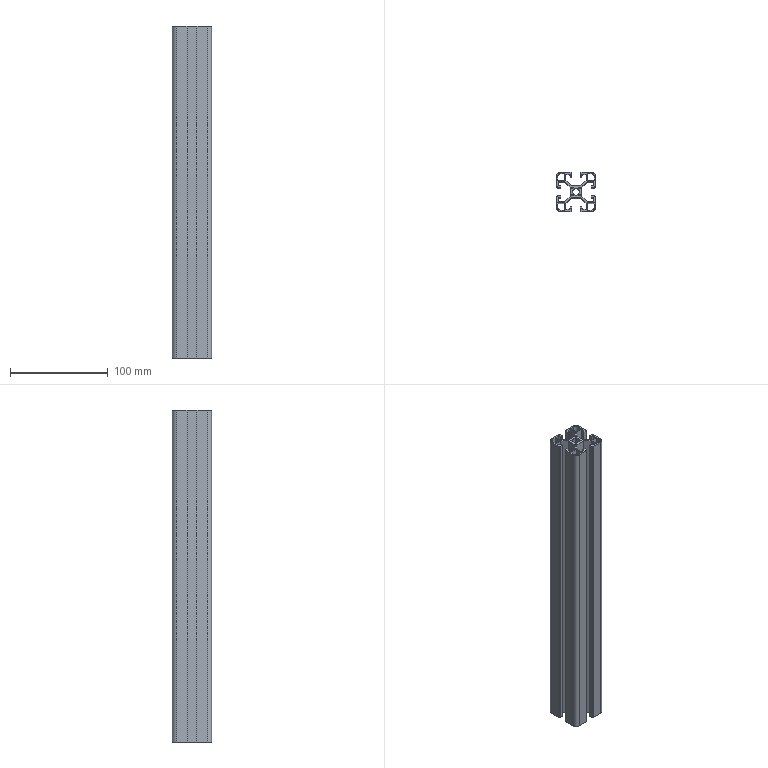Part | SolidWorks | features BaseBody 1, MoveFace 1 | 1 solid | 129 faces | box 40 x 40 x 339 mm | volume 146697 mm3 | plane 102 | cylinder 27 | commonest cylinder face diameters 2 x8 1.5 x6 6.8 x5 6.6 x4 9 x4